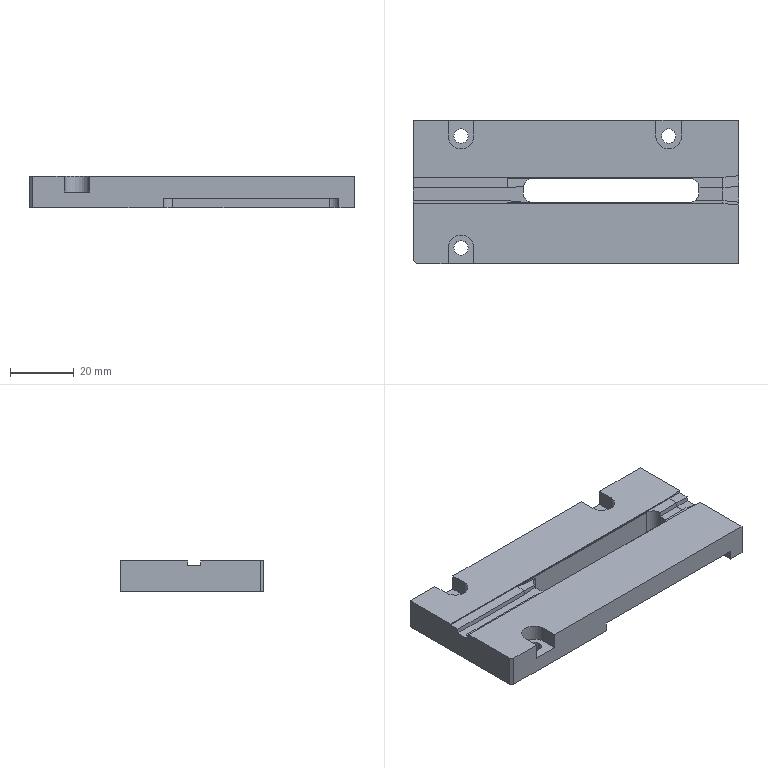Part | SolidWorks | features ICE 27, Fillet 10, Chamfer 8, HoleWzd 8, 3DProfileFeature 4, Cut 4, Extrusion 1 | 1 solid | 61 faces | box 102 x 45 x 10 mm | volume 38830 mm3 | plane 46 | cylinder 15 | commonest cylinder face diameters 4.5 x6 6 x6 8 x3